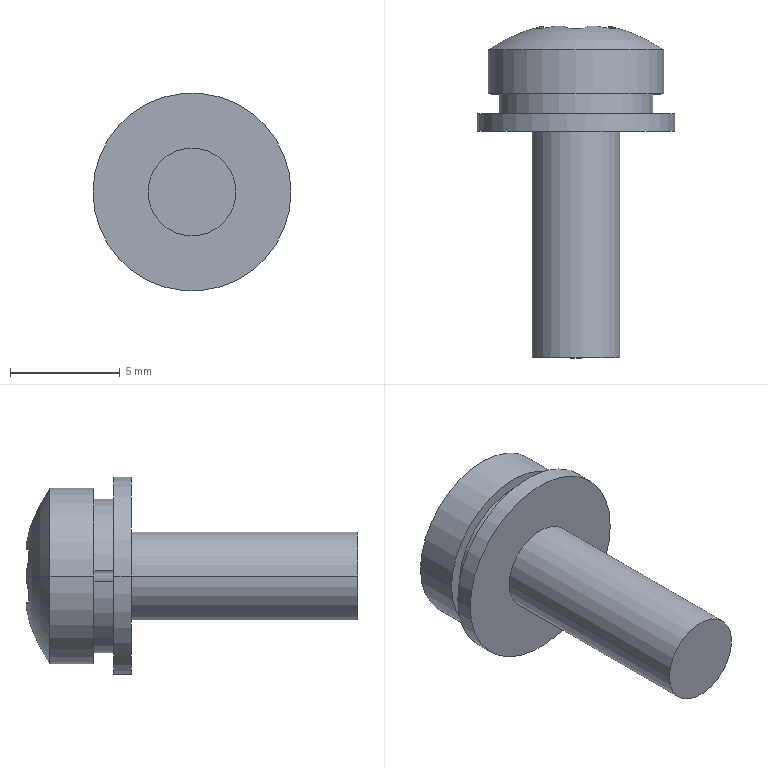Part | STEP file | LIB_68343071_M4X12 | 1 solid | 29 faces | box 9 x 15.088 x 9 mm | volume 332.967 mm3 | cylinder 20 | plane 7 | sphere 2 | commonest cylinder face diameters 0.992 x6 1.2 x6 4 x3 8 x2 9 x2 7 x1